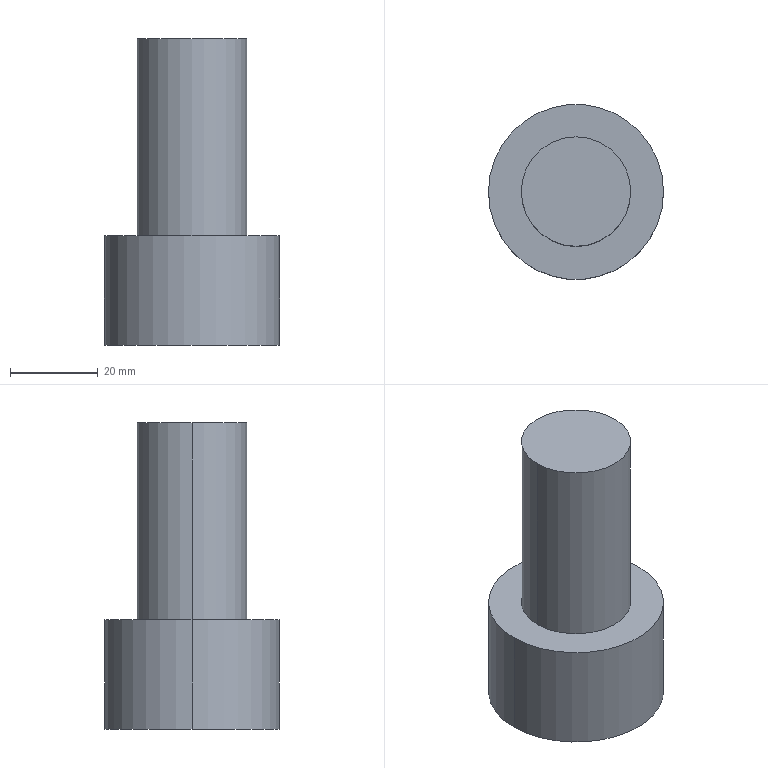Part | SolidWorks | features Extrusion 1, ICE 1 | 1 solid | 7 faces | box 40 x 40 x 70 mm | volume 53505 mm3 | cylinder 4 | plane 3 | commonest cylinder face diameters 25 x2 40 x2
STEP:
#1=CARTESIAN_POINT('',(12.5,0.,70.));
#2=VERTEX_POINT('',#1);
#3=CARTESIAN_POINT('',(-12.5,0.,70.));
#4=VERTEX_POINT('',#3);
#5=CARTESIAN_POINT('',(0.,0.,70.));
#6=DIRECTION('',(0.,0.,1.));
#7=DIRECTION('',(1.,0.,0.));
#8=AXIS2_PLACEMENT_3D('',#5,#6,#7);
#9=CIRCLE('',#8,12.5);
#10=EDGE_CURVE('',#2,#4,#9,.T.);
#11=ORIENTED_EDGE('',*,*,#10,.F.);
#12=CARTESIAN_POINT('',(12.5,0.,25.));
#13=VERTEX_POINT('',#12);
#14=CARTESIAN_POINT('',(12.5,0.,70.));
#15=DIRECTION('',(0.,0.,-1.));
#16=VECTOR('',#15,1000.);
#17=LINE('',#14,#16);
#18=EDGE_CURVE('',#2,#13,#17,.T.);
#19=ORIENTED_EDGE('',*,*,#18,.T.);
#20=CARTESIAN_POINT('',(-12.5,0.,25.));
#21=VERTEX_POINT('',#20);
#22=CARTESIAN_POINT('',(0.,0.,25.));
#23=DIRECTION('',(0.,0.,1.));
#24=DIRECTION('',(1.,0.,0.));
#25=AXIS2_PLACEMENT_3D('',#22,#23,#24);
#26=CIRCLE('',#25,12.5);
#27=EDGE_CURVE('',#13,#21,#26,.T.);
#28=ORIENTED_EDGE('',*,*,#27,.T.);
#29=CARTESIAN_POINT('',(-12.5,0.,70.));
#30=DIRECTION('',(0.,0.,-1.));
#31=VECTOR('',#30,1000.);
#32=LINE('',#29,#31);
#33=EDGE_CURVE('',#4,#21,#32,.T.);
#34=ORIENTED_EDGE('',*,*,#33,.F.);
#35=EDGE_LOOP('',(#11,#19,#28,#34));
#36=FACE_OUTER_BOUND('',#35,.T.);
#37=CARTESIAN_POINT('',(0.,0.,70.));
#38=DIRECTION('',(0.,0.,-1.));
#39=DIRECTION('',(-1.,0.,0.));
#40=AXIS2_PLACEMENT_3D('',#37,#38,#39);
#41=CYLINDRICAL_SURFACE('',#40,12.5);
#42=ADVANCED_FACE('',(#36),#41,.T.);
#43=CARTESIAN_POINT('',(20.,0.,25.));
#44=VERTEX_POINT('',#43);
#45=CARTESIAN_POINT('',(-20.,0.,25.));
#46=VERTEX_POINT('',#45);
#47=CARTESIAN_POINT('',(0.,0.,25.));
#48=DIRECTION('',(0.,0.,1.));
#49=DIRECTION('',(1.,0.,0.));
#50=AXIS2_PLACEMENT_3D('',#47,#48,#49);
#51=CIRCLE('',#50,20.);
#52=EDGE_CURVE('',#44,#46,#51,.T.);
#53=ORIENTED_EDGE('',*,*,#52,.F.);
#54=CARTESIAN_POINT('',(20.,0.,0.));
#55=VERTEX_POINT('',#54);
#56=CARTESIAN_POINT('',(20.,0.,25.));
#57=DIRECTION('',(0.,0.,-1.));
#58=VECTOR('',#57,1000.);
#59=LINE('',#56,#58);
#60=EDGE_CURVE('',#44,#55,#59,.T.);
#61=ORIENTED_EDGE('',*,*,#60,.T.);
#62=CARTESIAN_POINT('',(-20.,0.,0.));
#63=VERTEX_POINT('',#62);
#64=CARTESIAN_POINT('',(0.,0.,0.));
#65=DIRECTION('',(0.,0.,1.));
#66=DIRECTION('',(1.,0.,0.));
#67=AXIS2_PLACEMENT_3D('',#64,#65,#66);
#68=CIRCLE('',#67,20.);
#69=EDGE_CURVE('',#55,#63,#68,.T.);
#70=ORIENTED_EDGE('',*,*,#69,.T.);
#71=CARTESIAN_POINT('',(-20.,0.,25.));
#72=DIRECTION('',(0.,0.,-1.));
#73=VECTOR('',#72,1000.);
#74=LINE('',#71,#73);
#75=EDGE_CURVE('',#46,#63,#74,.T.);
#76=ORIENTED_EDGE('',*,*,#75,.F.);
#77=EDGE_LOOP('',(#53,#61,#70,#76));
#78=FACE_OUTER_BOUND('',#77,.T.);
#79=CARTESIAN_POINT('',(0.,0.,25.));
#80=DIRECTION('',(0.,0.,-1.));
#81=DIRECTION('',(-1.,0.,0.));
#82=AXIS2_PLACEMENT_3D('',#79,#80,#81);
#83=CYLINDRICAL_SURFACE('',#82,20.);
#84=ADVANCED_FACE('',(#78),#83,.T.);
#85=ORIENTED_EDGE('',*,*,#60,.F.);
#86=CARTESIAN_POINT('',(0.,0.,25.));
#87=DIRECTION('',(0.,0.,1.));
#88=DIRECTION('',(1.,0.,0.));
#89=AXIS2_PLACEMENT_3D('',#86,#87,#88);
#90=CIRCLE('',#89,20.);
#91=EDGE_CURVE('',#46,#44,#90,.T.);
#92=ORIENTED_EDGE('',*,*,#91,.F.);
#93=ORIENTED_EDGE('',*,*,#75,.T.);
#94=CARTESIAN_POINT('',(0.,0.,0.));
#95=DIRECTION('',(0.,0.,1.));
#96=DIRECTION('',(1.,0.,0.));
#97=AXIS2_PLACEMENT_3D('',#94,#95,#96);
#98=CIRCLE('',#97,20.);
#99=EDGE_CURVE('',#63,#55,#98,.T.);
#100=ORIENTED_EDGE('',*,*,#99,.T.);
#101=EDGE_LOOP('',(#85,#92,#93,#100));
#102=FACE_OUTER_BOUND('',#101,.T.);
#103=CARTESIAN_POINT('',(0.,0.,25.));
#104=DIRECTION('',(0.,0.,-1.));
#105=DIRECTION('',(-1.,0.,0.));
#106=AXIS2_PLACEMENT_3D('',#103,#104,#105);
#107=CYLINDRICAL_SURFACE('',#106,20.);
#108=ADVANCED_FACE('',(#102),#107,.T.);
#109=CARTESIAN_POINT('',(0.,0.,25.));
#110=DIRECTION('',(0.,0.,1.));
#111=DIRECTION('',(1.,0.,0.));
#112=AXIS2_PLACEMENT_3D('',#109,#110,#111);
#113=CIRCLE('',#112,12.5);
#114=EDGE_CURVE('',#21,#13,#113,.T.);
#115=ORIENTED_EDGE('',*,*,#114,.F.);
#116=ORIENTED_EDGE('',*,*,#27,.F.);
#117=EDGE_LOOP('',(#115,#116));
#118=FACE_BOUND('',#117,.T.);
#119=ORIENTED_EDGE('',*,*,#91,.T.);
#120=ORIENTED_EDGE('',*,*,#52,.T.);
#121=EDGE_LOOP('',(#119,#120));
#122=FACE_OUTER_BOUND('',#121,.T.);
#123=CARTESIAN_POINT('',(0.,0.,25.));
#124=DIRECTION('',(0.,0.,1.));
#125=DIRECTION('',(1.,0.,0.));
#126=AXIS2_PLACEMENT_3D('',#123,#124,#125);
#127=PLANE('',#126);
#128=ADVANCED_FACE('',(#118,#122),#127,.T.);
#129=ORIENTED_EDGE('',*,*,#99,.F.);
#130=ORIENTED_EDGE('',*,*,#69,.F.);
#131=EDGE_LOOP('',(#129,#130));
#132=FACE_OUTER_BOUND('',#131,.T.);
#133=CARTESIAN_POINT('',(0.,0.,0.));
#134=DIRECTION('',(0.,0.,1.));
#135=DIRECTION('',(1.,0.,0.));
#136=AXIS2_PLACEMENT_3D('',#133,#134,#135);
#137=PLANE('',#136);
#138=ADVANCED_FACE('',(#132),#137,.F.);
#139=ORIENTED_EDGE('',*,*,#18,.F.);
#140=CARTESIAN_POINT('',(0.,0.,70.));
#141=DIRECTION('',(0.,0.,1.));
#142=DIRECTION('',(1.,0.,0.));
#143=AXIS2_PLACEMENT_3D('',#140,#141,#142);
#144=CIRCLE('',#143,12.5);
#145=EDGE_CURVE('',#4,#2,#144,.T.);
#146=ORIENTED_EDGE('',*,*,#145,.F.);
#147=ORIENTED_EDGE('',*,*,#33,.T.);
#148=ORIENTED_EDGE('',*,*,#114,.T.);
#149=EDGE_LOOP('',(#139,#146,#147,#148));
#150=FACE_OUTER_BOUND('',#149,.T.);
#151=CARTESIAN_POINT('',(0.,0.,70.));
#152=DIRECTION('',(0.,0.,-1.));
#153=DIRECTION('',(-1.,0.,0.));
#154=AXIS2_PLACEMENT_3D('',#151,#152,#153);
#155=CYLINDRICAL_SURFACE('',#154,12.5);
#156=ADVANCED_FACE('',(#150),#155,.T.);
#157=ORIENTED_EDGE('',*,*,#145,.T.);
#158=ORIENTED_EDGE('',*,*,#10,.T.);
#159=EDGE_LOOP('',(#157,#158));
#160=FACE_OUTER_BOUND('',#159,.T.);
#161=CARTESIAN_POINT('',(0.,0.,70.));
#162=DIRECTION('',(0.,0.,1.));
#163=DIRECTION('',(1.,0.,0.));
#164=AXIS2_PLACEMENT_3D('',#161,#162,#163);
#165=PLANE('',#164);
#166=ADVANCED_FACE('',(#160),#165,.T.);
#167=CLOSED_SHELL('',(#42,#84,#108,#128,#138,#156,#166));
#168=MANIFOLD_SOLID_BREP('',#167);
#169=CARTESIAN_POINT('',(0.,0.,0.));
#170=DIRECTION('',(0.,0.,1.));
#171=DIRECTION('',(1.,0.,0.));
#172=AXIS2_PLACEMENT_3D('',#169,#170,#171);
#173=(LENGTH_UNIT()NAMED_UNIT(*)SI_UNIT(.MILLI.,.METRE.));
#174=UNCERTAINTY_MEASURE_WITH_UNIT(LENGTH_MEASURE(0.00001),#173,'','');
#175=(NAMED_UNIT(*)PLANE_ANGLE_UNIT()SI_UNIT($,.RADIAN.));
#176=(NAMED_UNIT(*)SI_UNIT($,.STERADIAN.)SOLID_ANGLE_UNIT());
#177=(GEOMETRIC_REPRESENTATION_CONTEXT(3)GLOBAL_UNCERTAINTY_ASSIGNED_CONTEXT((#174))GLOBAL_UNIT_ASSIGNED_CONTEXT((#173,#175,#176))REPRESENTATION_CONTEXT('',''));
#178=ADVANCED_BREP_SHAPE_REPRESENTATION('',(#168,#172),#177);